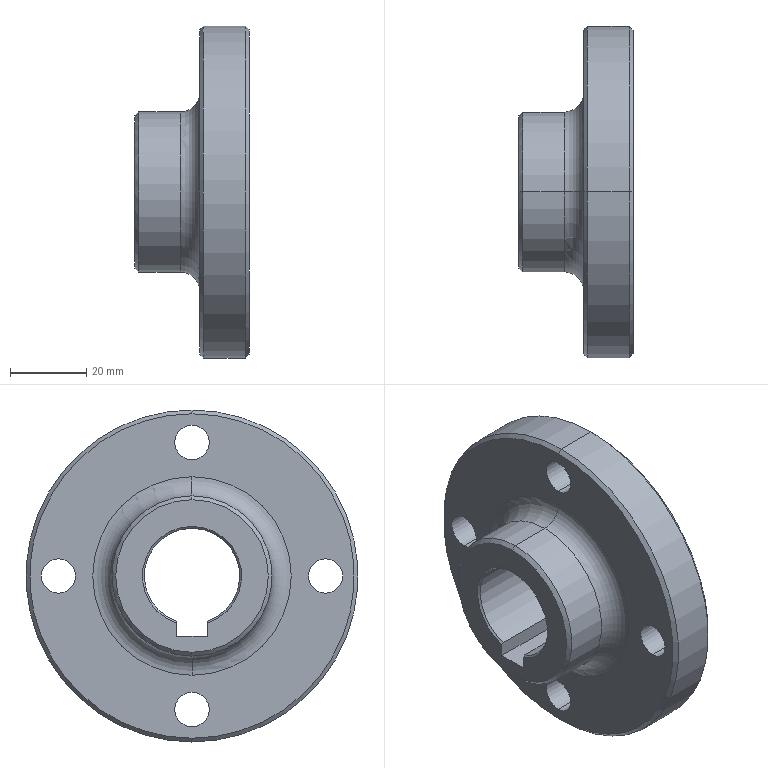Part | SolidWorks | features Chamfer 3, ICE 2, Fillet 1, Revolution 1 | 1 solid | 31 faces | box 30 x 87 x 87 mm | volume 82347 mm3 | cylinder 14 | cone 9 | plane 6 | torus 2 | commonest cylinder face diameters 9 x8 25 x2 42 x2 87 x2
STEP:
#1=CARTESIAN_POINT('',(30.,0.,-39.5));
#2=VERTEX_POINT('',#1);
#3=CARTESIAN_POINT('',(30.,0.,-30.5));
#4=VERTEX_POINT('',#3);
#5=CARTESIAN_POINT('',(30.,0.,-35.));
#6=DIRECTION('',(-1.,0.,0.));
#7=DIRECTION('',(0.,0.,1.));
#8=AXIS2_PLACEMENT_3D('',#5,#6,#7);
#9=CIRCLE('',#8,4.5);
#10=EDGE_CURVE('',#2,#4,#9,.T.);
#11=ORIENTED_EDGE('',*,*,#10,.F.);
#12=CARTESIAN_POINT('',(17.,0.,-39.5));
#13=VERTEX_POINT('',#12);
#14=CARTESIAN_POINT('',(37.,0.,-39.5));
#15=DIRECTION('',(-1.,0.,0.));
#16=VECTOR('',#15,1000.);
#17=LINE('',#14,#16);
#18=EDGE_CURVE('',#2,#13,#17,.T.);
#19=ORIENTED_EDGE('',*,*,#18,.T.);
#20=CARTESIAN_POINT('',(17.,0.,-30.5));
#21=VERTEX_POINT('',#20);
#22=CARTESIAN_POINT('',(17.,0.,-35.));
#23=DIRECTION('',(-1.,0.,0.));
#24=DIRECTION('',(0.,0.,1.));
#25=AXIS2_PLACEMENT_3D('',#22,#23,#24);
#26=CIRCLE('',#25,4.5);
#27=EDGE_CURVE('',#13,#21,#26,.T.);
#28=ORIENTED_EDGE('',*,*,#27,.T.);
#29=CARTESIAN_POINT('',(37.,0.,-30.5));
#30=DIRECTION('',(-1.,0.,0.));
#31=VECTOR('',#30,1000.);
#32=LINE('',#29,#31);
#33=EDGE_CURVE('',#4,#21,#32,.T.);
#34=ORIENTED_EDGE('',*,*,#33,.F.);
#35=EDGE_LOOP('',(#11,#19,#28,#34));
#36=FACE_OUTER_BOUND('',#35,.T.);
#37=CARTESIAN_POINT('',(37.,0.,-35.));
#38=DIRECTION('',(-1.,0.,0.));
#39=DIRECTION('',(0.,0.,1.));
#40=AXIS2_PLACEMENT_3D('',#37,#38,#39);
#41=CYLINDRICAL_SURFACE('',#40,4.5);
#42=ADVANCED_FACE('',(#36),#41,.F.);
#43=CARTESIAN_POINT('',(30.,35.,-4.5));
#44=VERTEX_POINT('',#43);
#45=CARTESIAN_POINT('',(30.,35.,4.5));
#46=VERTEX_POINT('',#45);
#47=CARTESIAN_POINT('',(30.,35.,0.));
#48=DIRECTION('',(-1.,0.,0.));
#49=DIRECTION('',(0.,0.,1.));
#50=AXIS2_PLACEMENT_3D('',#47,#48,#49);
#51=CIRCLE('',#50,4.5);
#52=EDGE_CURVE('',#44,#46,#51,.T.);
#53=ORIENTED_EDGE('',*,*,#52,.F.);
#54=CARTESIAN_POINT('',(17.,35.,-4.5));
#55=VERTEX_POINT('',#54);
#56=CARTESIAN_POINT('',(37.,35.,-4.5));
#57=DIRECTION('',(-1.,0.,0.));
#58=VECTOR('',#57,1000.);
#59=LINE('',#56,#58);
#60=EDGE_CURVE('',#44,#55,#59,.T.);
#61=ORIENTED_EDGE('',*,*,#60,.T.);
#62=CARTESIAN_POINT('',(17.,35.,4.5));
#63=VERTEX_POINT('',#62);
#64=CARTESIAN_POINT('',(17.,35.,0.));
#65=DIRECTION('',(-1.,0.,0.));
#66=DIRECTION('',(0.,0.,1.));
#67=AXIS2_PLACEMENT_3D('',#64,#65,#66);
#68=CIRCLE('',#67,4.5);
#69=EDGE_CURVE('',#55,#63,#68,.T.);
#70=ORIENTED_EDGE('',*,*,#69,.T.);
#71=CARTESIAN_POINT('',(37.,35.,4.5));
#72=DIRECTION('',(-1.,0.,0.));
#73=VECTOR('',#72,1000.);
#74=LINE('',#71,#73);
#75=EDGE_CURVE('',#46,#63,#74,.T.);
#76=ORIENTED_EDGE('',*,*,#75,.F.);
#77=EDGE_LOOP('',(#53,#61,#70,#76));
#78=FACE_OUTER_BOUND('',#77,.T.);
#79=CARTESIAN_POINT('',(37.,35.,0.));
#80=DIRECTION('',(-1.,0.,0.));
#81=DIRECTION('',(0.,0.,1.));
#82=AXIS2_PLACEMENT_3D('',#79,#80,#81);
#83=CYLINDRICAL_SURFACE('',#82,4.5);
#84=ADVANCED_FACE('',(#78),#83,.F.);
#85=CARTESIAN_POINT('',(30.,-35.,-4.5));
#86=VERTEX_POINT('',#85);
#87=CARTESIAN_POINT('',(30.,-35.,4.5));
#88=VERTEX_POINT('',#87);
#89=CARTESIAN_POINT('',(30.,-35.,0.));
#90=DIRECTION('',(-1.,0.,0.));
#91=DIRECTION('',(0.,0.,1.));
#92=AXIS2_PLACEMENT_3D('',#89,#90,#91);
#93=CIRCLE('',#92,4.5);
#94=EDGE_CURVE('',#86,#88,#93,.T.);
#95=ORIENTED_EDGE('',*,*,#94,.F.);
#96=CARTESIAN_POINT('',(17.,-35.,-4.5));
#97=VERTEX_POINT('',#96);
#98=CARTESIAN_POINT('',(37.,-35.,-4.5));
#99=DIRECTION('',(-1.,0.,0.));
#100=VECTOR('',#99,1000.);
#101=LINE('',#98,#100);
#102=EDGE_CURVE('',#86,#97,#101,.T.);
#103=ORIENTED_EDGE('',*,*,#102,.T.);
#104=CARTESIAN_POINT('',(17.,-35.,4.5));
#105=VERTEX_POINT('',#104);
#106=CARTESIAN_POINT('',(17.,-35.,0.));
#107=DIRECTION('',(-1.,0.,0.));
#108=DIRECTION('',(0.,0.,1.));
#109=AXIS2_PLACEMENT_3D('',#106,#107,#108);
#110=CIRCLE('',#109,4.5);
#111=EDGE_CURVE('',#97,#105,#110,.T.);
#112=ORIENTED_EDGE('',*,*,#111,.T.);
#113=CARTESIAN_POINT('',(37.,-35.,4.5));
#114=DIRECTION('',(-1.,0.,0.));
#115=VECTOR('',#114,1000.);
#116=LINE('',#113,#115);
#117=EDGE_CURVE('',#88,#105,#116,.T.);
#118=ORIENTED_EDGE('',*,*,#117,.F.);
#119=EDGE_LOOP('',(#95,#103,#112,#118));
#120=FACE_OUTER_BOUND('',#119,.T.);
#121=CARTESIAN_POINT('',(37.,-35.,0.));
#122=DIRECTION('',(-1.,0.,0.));
#123=DIRECTION('',(0.,0.,1.));
#124=AXIS2_PLACEMENT_3D('',#121,#122,#123);
#125=CYLINDRICAL_SURFACE('',#124,4.5);
#126=ADVANCED_FACE('',(#120),#125,.F.);
#127=CARTESIAN_POINT('',(30.,0.,30.5));
#128=VERTEX_POINT('',#127);
#129=CARTESIAN_POINT('',(30.,0.,39.5));
#130=VERTEX_POINT('',#129);
#131=CARTESIAN_POINT('',(30.,0.,35.));
#132=DIRECTION('',(-1.,0.,0.));
#133=DIRECTION('',(0.,0.,1.));
#134=AXIS2_PLACEMENT_3D('',#131,#132,#133);
#135=CIRCLE('',#134,4.5);
#136=EDGE_CURVE('',#128,#130,#135,.T.);
#137=ORIENTED_EDGE('',*,*,#136,.F.);
#138=CARTESIAN_POINT('',(17.,0.,30.5));
#139=VERTEX_POINT('',#138);
#140=CARTESIAN_POINT('',(37.,0.,30.5));
#141=DIRECTION('',(-1.,0.,0.));
#142=VECTOR('',#141,1000.);
#143=LINE('',#140,#142);
#144=EDGE_CURVE('',#128,#139,#143,.T.);
#145=ORIENTED_EDGE('',*,*,#144,.T.);
#146=CARTESIAN_POINT('',(17.,0.,39.5));
#147=VERTEX_POINT('',#146);
#148=CARTESIAN_POINT('',(17.,0.,35.));
#149=DIRECTION('',(-1.,0.,0.));
#150=DIRECTION('',(0.,0.,1.));
#151=AXIS2_PLACEMENT_3D('',#148,#149,#150);
#152=CIRCLE('',#151,4.5);
#153=EDGE_CURVE('',#139,#147,#152,.T.);
#154=ORIENTED_EDGE('',*,*,#153,.T.);
#155=CARTESIAN_POINT('',(37.,0.,39.5));
#156=DIRECTION('',(-1.,0.,0.));
#157=VECTOR('',#156,1000.);
#158=LINE('',#155,#157);
#159=EDGE_CURVE('',#130,#147,#158,.T.);
#160=ORIENTED_EDGE('',*,*,#159,.F.);
#161=EDGE_LOOP('',(#137,#145,#154,#160));
#162=FACE_OUTER_BOUND('',#161,.T.);
#163=CARTESIAN_POINT('',(37.,0.,35.));
#164=DIRECTION('',(-1.,0.,0.));
#165=DIRECTION('',(0.,0.,1.));
#166=AXIS2_PLACEMENT_3D('',#163,#164,#165);
#167=CYLINDRICAL_SURFACE('',#166,4.5);
#168=ADVANCED_FACE('',(#162),#167,.F.);
#169=CARTESIAN_POINT('',(17.,0.,42.5));
#170=VERTEX_POINT('',#169);
#171=CARTESIAN_POINT('',(17.,0.,-42.5));
#172=VERTEX_POINT('',#171);
#173=CARTESIAN_POINT('',(17.,0.,0.));
#174=DIRECTION('',(-1.,0.,0.));
#175=DIRECTION('',(0.,0.,-1.));
#176=AXIS2_PLACEMENT_3D('',#173,#174,#175);
#177=CIRCLE('',#176,42.5);
#178=EDGE_CURVE('',#170,#172,#177,.T.);
#179=ORIENTED_EDGE('',*,*,#178,.F.);
#180=CARTESIAN_POINT('',(18.,0.,43.5));
#181=VERTEX_POINT('',#180);
#182=CARTESIAN_POINT('',(17.,0.,42.5));
#183=DIRECTION('',(0.7071,0.,0.7071));
#184=VECTOR('',#183,1000.);
#185=LINE('',#182,#184);
#186=EDGE_CURVE('',#170,#181,#185,.T.);
#187=ORIENTED_EDGE('',*,*,#186,.T.);
#188=CARTESIAN_POINT('',(18.,0.,-43.5));
#189=VERTEX_POINT('',#188);
#190=CARTESIAN_POINT('',(18.,0.,0.));
#191=DIRECTION('',(1.,0.,0.));
#192=DIRECTION('',(0.,0.,-1.));
#193=AXIS2_PLACEMENT_3D('',#190,#191,#192);
#194=CIRCLE('',#193,43.5);
#195=EDGE_CURVE('',#189,#181,#194,.T.);
#196=ORIENTED_EDGE('',*,*,#195,.F.);
#197=CARTESIAN_POINT('',(17.,0.,-42.5));
#198=DIRECTION('',(0.7071,0.,-0.7071));
#199=VECTOR('',#198,1000.);
#200=LINE('',#197,#199);
#201=EDGE_CURVE('',#172,#189,#200,.T.);
#202=ORIENTED_EDGE('',*,*,#201,.F.);
#203=EDGE_LOOP('',(#179,#187,#196,#202));
#204=FACE_OUTER_BOUND('',#203,.T.);
#205=CARTESIAN_POINT('',(17.,0.,0.));
#206=DIRECTION('',(1.,0.,0.));
#207=DIRECTION('',(0.,0.,-1.));
#208=AXIS2_PLACEMENT_3D('',#205,#206,#207);
#209=CONICAL_SURFACE('',#208,42.5,0.7854);
#210=ADVANCED_FACE('',(#204),#209,.T.);
#211=CARTESIAN_POINT('',(30.,0.,-42.5));
#212=VERTEX_POINT('',#211);
#213=CARTESIAN_POINT('',(30.,0.,42.5));
#214=VERTEX_POINT('',#213);
#215=CARTESIAN_POINT('',(30.,0.,0.));
#216=DIRECTION('',(1.,0.,0.));
#217=DIRECTION('',(0.,0.,1.));
#218=AXIS2_PLACEMENT_3D('',#215,#216,#217);
#219=CIRCLE('',#218,42.5);
#220=EDGE_CURVE('',#212,#214,#219,.T.);
#221=ORIENTED_EDGE('',*,*,#220,.F.);
#222=CARTESIAN_POINT('',(29.,0.,-43.5));
#223=VERTEX_POINT('',#222);
#224=CARTESIAN_POINT('',(29.,0.,-43.5));
#225=DIRECTION('',(-0.7071,0.,-0.7071));
#226=VECTOR('',#225,1000.);
#227=LINE('',#224,#226);
#228=EDGE_CURVE('',#212,#223,#227,.T.);
#229=ORIENTED_EDGE('',*,*,#228,.T.);
#230=CARTESIAN_POINT('',(29.,0.,43.5));
#231=VERTEX_POINT('',#230);
#232=CARTESIAN_POINT('',(29.,0.,0.));
#233=DIRECTION('',(-1.,0.,0.));
#234=DIRECTION('',(0.,0.,1.));
#235=AXIS2_PLACEMENT_3D('',#232,#233,#234);
#236=CIRCLE('',#235,43.5);
#237=EDGE_CURVE('',#231,#223,#236,.T.);
#238=ORIENTED_EDGE('',*,*,#237,.F.);
#239=CARTESIAN_POINT('',(29.,0.,43.5));
#240=DIRECTION('',(-0.7071,0.,0.7071));
#241=VECTOR('',#240,1000.);
#242=LINE('',#239,#241);
#243=EDGE_CURVE('',#214,#231,#242,.T.);
#244=ORIENTED_EDGE('',*,*,#243,.F.);
#245=EDGE_LOOP('',(#221,#229,#238,#244));
#246=FACE_OUTER_BOUND('',#245,.T.);
#247=CARTESIAN_POINT('',(29.,0.,0.));
#248=DIRECTION('',(-1.,0.,0.));
#249=DIRECTION('',(0.,0.,1.));
#250=AXIS2_PLACEMENT_3D('',#247,#248,#249);
#251=CONICAL_SURFACE('',#250,43.5,0.7854);
#252=ADVANCED_FACE('',(#246),#251,.T.);
#253=CARTESIAN_POINT('',(17.,0.,26.));
#254=VERTEX_POINT('',#253);
#255=CARTESIAN_POINT('',(17.,0.,-26.));
#256=VERTEX_POINT('',#255);
#257=CARTESIAN_POINT('',(17.,0.,0.));
#258=DIRECTION('',(1.,0.,0.));
#259=DIRECTION('',(0.,0.,-1.));
#260=AXIS2_PLACEMENT_3D('',#257,#258,#259);
#261=CIRCLE('',#260,26.);
#262=EDGE_CURVE('',#254,#256,#261,.T.);
#263=ORIENTED_EDGE('',*,*,#262,.F.);
#264=CARTESIAN_POINT('',(12.,0.,21.));
#265=VERTEX_POINT('',#264);
#266=CARTESIAN_POINT('',(12.,0.,26.));
#267=DIRECTION('',(0.,1.,0.));
#268=DIRECTION('',(0.,0.,1.));
#269=AXIS2_PLACEMENT_3D('',#266,#267,#268);
#270=CIRCLE('',#269,5.);
#271=EDGE_CURVE('',#254,#265,#270,.T.);
#272=ORIENTED_EDGE('',*,*,#271,.T.);
#273=CARTESIAN_POINT('',(12.,0.,-21.));
#274=VERTEX_POINT('',#273);
#275=CARTESIAN_POINT('',(12.,0.,0.));
#276=DIRECTION('',(-1.,0.,0.));
#277=DIRECTION('',(0.,0.,-1.));
#278=AXIS2_PLACEMENT_3D('',#275,#276,#277);
#279=CIRCLE('',#278,21.);
#280=EDGE_CURVE('',#274,#265,#279,.T.);
#281=ORIENTED_EDGE('',*,*,#280,.F.);
#282=CARTESIAN_POINT('',(12.,0.,-26.));
#283=DIRECTION('',(0.,-1.,0.));
#284=DIRECTION('',(0.,0.,-1.));
#285=AXIS2_PLACEMENT_3D('',#282,#283,#284);
#286=CIRCLE('',#285,5.);
#287=EDGE_CURVE('',#256,#274,#286,.T.);
#288=ORIENTED_EDGE('',*,*,#287,.F.);
#289=EDGE_LOOP('',(#263,#272,#281,#288));
#290=FACE_OUTER_BOUND('',#289,.T.);
#291=CARTESIAN_POINT('',(12.,0.,0.));
#292=DIRECTION('',(1.,0.,0.));
#293=DIRECTION('',(0.,0.,-1.));
#294=AXIS2_PLACEMENT_3D('',#291,#292,#293);
#295=TOROIDAL_SURFACE('',#294,26.,5.);
#296=ADVANCED_FACE('',(#290),#295,.F.);
#297=CARTESIAN_POINT('',(0.5,0.,12.5));
#298=VERTEX_POINT('',#297);
#299=CARTESIAN_POINT('',(0.5,4.,-11.843));
#300=VERTEX_POINT('',#299);
#301=CARTESIAN_POINT('',(0.5,0.,0.));
#302=DIRECTION('',(-1.,0.,0.));
#303=DIRECTION('',(0.,0.,-1.));
#304=AXIS2_PLACEMENT_3D('',#301,#302,#303);
#305=CIRCLE('',#304,12.5);
#306=EDGE_CURVE('',#298,#300,#305,.T.);
#307=ORIENTED_EDGE('',*,*,#306,.F.);
#308=CARTESIAN_POINT('',(0.,0.,13.));
#309=VERTEX_POINT('',#308);
#310=CARTESIAN_POINT('',(0.5,0.,12.5));
#311=DIRECTION('',(-0.7071,0.,0.7071));
#312=VECTOR('',#311,1000.);
#313=LINE('',#310,#312);
#314=EDGE_CURVE('',#298,#309,#313,.T.);
#315=ORIENTED_EDGE('',*,*,#314,.T.);
#316=CARTESIAN_POINT('',(0.,4.,-12.369));
#317=VERTEX_POINT('',#316);
#318=CARTESIAN_POINT('',(0.,0.,0.));
#319=DIRECTION('',(1.,0.,0.));
#320=DIRECTION('',(0.,0.,-1.));
#321=AXIS2_PLACEMENT_3D('',#318,#319,#320);
#322=CIRCLE('',#321,13.);
#323=EDGE_CURVE('',#317,#309,#322,.T.);
#324=ORIENTED_EDGE('',*,*,#323,.F.);
#325=CARTESIAN_POINT('',(0.5,4.,-11.843));
#326=CARTESIAN_POINT('',(0.3335,4.,-12.018));
#327=CARTESIAN_POINT('',(0.1669,4.,-12.194));
#328=CARTESIAN_POINT('',(0.,4.,-12.369));
#329=B_SPLINE_CURVE_WITH_KNOTS('',3,(#325,#326,#327,#328),.UNSPECIFIED.,.F.,.F.,(4,4),(0.00787,0.008596),.UNSPECIFIED.);
#330=EDGE_CURVE('',#300,#317,#329,.T.);
#331=ORIENTED_EDGE('',*,*,#330,.F.);
#332=EDGE_LOOP('',(#307,#315,#324,#331));
#333=FACE_OUTER_BOUND('',#332,.T.);
#334=CARTESIAN_POINT('',(0.5,0.,0.));
#335=DIRECTION('',(-1.,0.,0.));
#336=DIRECTION('',(0.,0.,1.));
#337=AXIS2_PLACEMENT_3D('',#334,#335,#336);
#338=CONICAL_SURFACE('',#337,12.5,0.7854);
#339=ADVANCED_FACE('',(#333),#338,.F.);
#340=CARTESIAN_POINT('',(0.,0.,20.));
#341=VERTEX_POINT('',#340);
#342=CARTESIAN_POINT('',(0.,0.,-20.));
#343=VERTEX_POINT('',#342);
#344=CARTESIAN_POINT('',(0.,0.,0.));
#345=DIRECTION('',(-1.,0.,0.));
#346=DIRECTION('',(0.,0.,-1.));
#347=AXIS2_PLACEMENT_3D('',#344,#345,#346);
#348=CIRCLE('',#347,20.);
#349=EDGE_CURVE('',#341,#343,#348,.T.);
#350=ORIENTED_EDGE('',*,*,#349,.F.);
#351=CARTESIAN_POINT('',(1.,0.,21.));
#352=VERTEX_POINT('',#351);
#353=CARTESIAN_POINT('',(0.,0.,20.));
#354=DIRECTION('',(0.7071,0.,0.7071));
#355=VECTOR('',#354,1000.);
#356=LINE('',#353,#355);
#357=EDGE_CURVE('',#341,#352,#356,.T.);
#358=ORIENTED_EDGE('',*,*,#357,.T.);
#359=CARTESIAN_POINT('',(1.,0.,-21.));
#360=VERTEX_POINT('',#359);
#361=CARTESIAN_POINT('',(1.,0.,0.));
#362=DIRECTION('',(1.,0.,0.));
#363=DIRECTION('',(0.,0.,-1.));
#364=AXIS2_PLACEMENT_3D('',#361,#362,#363);
#365=CIRCLE('',#364,21.);
#366=EDGE_CURVE('',#360,#352,#365,.T.);
#367=ORIENTED_EDGE('',*,*,#366,.F.);
#368=CARTESIAN_POINT('',(0.,0.,-20.));
#369=DIRECTION('',(0.7071,0.,-0.7071));
#370=VECTOR('',#369,1000.);
#371=LINE('',#368,#370);
#372=EDGE_CURVE('',#343,#360,#371,.T.);
#373=ORIENTED_EDGE('',*,*,#372,.F.);
#374=EDGE_LOOP('',(#350,#358,#367,#373));
#375=FACE_OUTER_BOUND('',#374,.T.);
#376=CARTESIAN_POINT('',(0.,0.,0.));
#377=DIRECTION('',(1.,0.,0.));
#378=DIRECTION('',(0.,0.,-1.));
#379=AXIS2_PLACEMENT_3D('',#376,#377,#378);
#380=CONICAL_SURFACE('',#379,20.,0.7854);
#381=ADVANCED_FACE('',(#375),#380,.T.);
#382=ORIENTED_EDGE('',*,*,#237,.T.);
#383=CARTESIAN_POINT('',(0.,0.,-43.5));
#384=DIRECTION('',(-1.,0.,0.));
#385=VECTOR('',#384,1000.);
#386=LINE('',#383,#385);
#387=EDGE_CURVE('',#223,#189,#386,.T.);
#388=ORIENTED_EDGE('',*,*,#387,.T.);
#389=ORIENTED_EDGE('',*,*,#195,.T.);
#390=CARTESIAN_POINT('',(0.,0.,43.5));
#391=DIRECTION('',(-1.,0.,0.));
#392=VECTOR('',#391,1000.);
#393=LINE('',#390,#392);
#394=EDGE_CURVE('',#231,#181,#393,.T.);
#395=ORIENTED_EDGE('',*,*,#394,.F.);
#396=EDGE_LOOP('',(#382,#388,#389,#395));
#397=FACE_OUTER_BOUND('',#396,.T.);
#398=CARTESIAN_POINT('',(0.,0.,0.));
#399=DIRECTION('',(-1.,0.,0.));
#400=DIRECTION('',(0.,0.,1.));
#401=AXIS2_PLACEMENT_3D('',#398,#399,#400);
#402=CYLINDRICAL_SURFACE('',#401,43.5);
#403=ADVANCED_FACE('',(#397),#402,.T.);
#404=CARTESIAN_POINT('',(29.5,4.,-11.843));
#405=VERTEX_POINT('',#404);
#406=CARTESIAN_POINT('',(29.5,0.,12.5));
#407=VERTEX_POINT('',#406);
#408=CARTESIAN_POINT('',(29.5,0.,0.));
#409=DIRECTION('',(1.,0.,0.));
#410=DIRECTION('',(0.,0.,1.));
#411=AXIS2_PLACEMENT_3D('',#408,#409,#410);
#412=CIRCLE('',#411,12.5);
#413=EDGE_CURVE('',#405,#407,#412,.T.);
#414=ORIENTED_EDGE('',*,*,#413,.T.);
#415=CARTESIAN_POINT('',(0.,0.,12.5));
#416=DIRECTION('',(-1.,0.,0.));
#417=VECTOR('',#416,1000.);
#418=LINE('',#415,#417);
#419=EDGE_CURVE('',#407,#298,#418,.T.);
#420=ORIENTED_EDGE('',*,*,#419,.T.);
#421=ORIENTED_EDGE('',*,*,#306,.T.);
#422=CARTESIAN_POINT('',(0.,4.,-11.843));
#423=DIRECTION('',(1.,0.,0.));
#424=VECTOR('',#423,1000.);
#425=LINE('',#422,#424);
#426=EDGE_CURVE('',#300,#405,#425,.T.);
#427=ORIENTED_EDGE('',*,*,#426,.T.);
#428=EDGE_LOOP('',(#414,#420,#421,#427));
#429=FACE_OUTER_BOUND('',#428,.T.);
#430=CARTESIAN_POINT('',(0.,0.,0.));
#431=DIRECTION('',(-1.,0.,0.));
#432=DIRECTION('',(0.,0.,1.));
#433=AXIS2_PLACEMENT_3D('',#430,#431,#432);
#434=CYLINDRICAL_SURFACE('',#433,12.5);
#435=ADVANCED_FACE('',(#429),#434,.F.);
#436=CARTESIAN_POINT('',(12.,0.,0.));
#437=DIRECTION('',(-1.,0.,0.));
#438=DIRECTION('',(0.,0.,-1.));
#439=AXIS2_PLACEMENT_3D('',#436,#437,#438);
#440=CIRCLE('',#439,21.);
#441=EDGE_CURVE('',#265,#274,#440,.T.);
#442=ORIENTED_EDGE('',*,*,#441,.T.);
#443=CARTESIAN_POINT('',(0.,0.,-21.));
#444=DIRECTION('',(-1.,0.,0.));
#445=VECTOR('',#444,1000.);
#446=LINE('',#443,#445);
#447=EDGE_CURVE('',#274,#360,#446,.T.);
#448=ORIENTED_EDGE('',*,*,#447,.T.);
#449=ORIENTED_EDGE('',*,*,#366,.T.);
#450=CARTESIAN_POINT('',(0.,0.,21.));
#451=DIRECTION('',(-1.,0.,0.));
#452=VECTOR('',#451,1000.);
#453=LINE('',#450,#452);
#454=EDGE_CURVE('',#265,#352,#453,.T.);
#455=ORIENTED_EDGE('',*,*,#454,.F.);
#456=EDGE_LOOP('',(#442,#448,#449,#455));
#457=FACE_OUTER_BOUND('',#456,.T.);
#458=CARTESIAN_POINT('',(0.,0.,0.));
#459=DIRECTION('',(-1.,0.,0.));
#460=DIRECTION('',(0.,0.,1.));
#461=AXIS2_PLACEMENT_3D('',#458,#459,#460);
#462=CYLINDRICAL_SURFACE('',#461,21.);
#463=ADVANCED_FACE('',(#457),#462,.T.);
#464=ORIENTED_EDGE('',*,*,#447,.F.);
#465=ORIENTED_EDGE('',*,*,#280,.T.);
#466=ORIENTED_EDGE('',*,*,#454,.T.);
#467=CARTESIAN_POINT('',(1.,0.,0.));
#468=DIRECTION('',(1.,0.,0.));
#469=DIRECTION('',(0.,0.,-1.));
#470=AXIS2_PLACEMENT_3D('',#467,#468,#469);
#471=CIRCLE('',#470,21.);
#472=EDGE_CURVE('',#352,#360,#471,.T.);
#473=ORIENTED_EDGE('',*,*,#472,.T.);
#474=EDGE_LOOP('',(#464,#465,#466,#473));
#475=FACE_OUTER_BOUND('',#474,.T.);
#476=CARTESIAN_POINT('',(0.,0.,0.));
#477=DIRECTION('',(-1.,0.,0.));
#478=DIRECTION('',(0.,0.,1.));
#479=AXIS2_PLACEMENT_3D('',#476,#477,#478);
#480=CYLINDRICAL_SURFACE('',#479,21.);
#481=ADVANCED_FACE('',(#475),#480,.T.);
#482=ORIENTED_EDGE('',*,*,#323,.T.);
#483=CARTESIAN_POINT('',(0.,-4.,-12.369));
#484=VERTEX_POINT('',#483);
#485=CARTESIAN_POINT('',(0.,0.,0.));
#486=DIRECTION('',(1.,0.,0.));
#487=DIRECTION('',(0.,0.,-1.));
#488=AXIS2_PLACEMENT_3D('',#485,#486,#487);
#489=CIRCLE('',#488,13.);
#490=EDGE_CURVE('',#309,#484,#489,.T.);
#491=ORIENTED_EDGE('',*,*,#490,.T.);
#492=CARTESIAN_POINT('',(0.,-4.,-15.8));
#493=VERTEX_POINT('',#492);
#494=CARTESIAN_POINT('',(0.,-4.,-15.8));
#495=DIRECTION('',(0.,0.,-1.));
#496=VECTOR('',#495,1000.);
#497=LINE('',#494,#496);
#498=EDGE_CURVE('',#484,#493,#497,.T.);
#499=ORIENTED_EDGE('',*,*,#498,.T.);
#500=CARTESIAN_POINT('',(0.,4.,-15.8));
#501=VERTEX_POINT('',#500);
#502=CARTESIAN_POINT('',(0.,4.,-15.8));
#503=DIRECTION('',(0.,1.,0.));
#504=VECTOR('',#503,1000.);
#505=LINE('',#502,#504);
#506=EDGE_CURVE('',#493,#501,#505,.T.);
#507=ORIENTED_EDGE('',*,*,#506,.T.);
#508=CARTESIAN_POINT('',(0.,4.,-15.8));
#509=DIRECTION('',(0.,0.,1.));
#510=VECTOR('',#509,1000.);
#511=LINE('',#508,#510);
#512=EDGE_CURVE('',#501,#317,#511,.T.);
#513=ORIENTED_EDGE('',*,*,#512,.T.);
#514=EDGE_LOOP('',(#482,#491,#499,#507,#513));
#515=FACE_BOUND('',#514,.T.);
#516=CARTESIAN_POINT('',(0.,0.,0.));
#517=DIRECTION('',(-1.,0.,0.));
#518=DIRECTION('',(0.,0.,-1.));
#519=AXIS2_PLACEMENT_3D('',#516,#517,#518);
#520=CIRCLE('',#519,20.);
#521=EDGE_CURVE('',#343,#341,#520,.T.);
#522=ORIENTED_EDGE('',*,*,#521,.T.);
#523=ORIENTED_EDGE('',*,*,#349,.T.);
#524=EDGE_LOOP('',(#522,#523));
#525=FACE_OUTER_BOUND('',#524,.T.);
#526=CARTESIAN_POINT('',(0.,12.5,0.));
#527=DIRECTION('',(1.,0.,0.));
#528=DIRECTION('',(0.,0.,-1.));
#529=AXIS2_PLACEMENT_3D('',#526,#527,#528);
#530=PLANE('',#529);
#531=ADVANCED_FACE('',(#515,#525),#530,.F.);
#532=ORIENTED_EDGE('',*,*,#419,.F.);
#533=CARTESIAN_POINT('',(29.5,-4.,-11.843));
#534=VERTEX_POINT('',#533);
#535=CARTESIAN_POINT('',(29.5,0.,0.));
#536=DIRECTION('',(1.,0.,0.));
#537=DIRECTION('',(0.,0.,1.));
#538=AXIS2_PLACEMENT_3D('',#535,#536,#537);
#539=CIRCLE('',#538,12.5);
#540=EDGE_CURVE('',#407,#534,#539,.T.);
#541=ORIENTED_EDGE('',*,*,#540,.T.);
#542=CARTESIAN_POINT('',(0.5,-4.,-11.843));
#543=VERTEX_POINT('',#542);
#544=CARTESIAN_POINT('',(0.,-4.,-11.843));
#545=DIRECTION('',(-1.,0.,0.));
#546=VECTOR('',#545,1000.);
#547=LINE('',#544,#546);
#548=EDGE_CURVE('',#534,#543,#547,.T.);
#549=ORIENTED_EDGE('',*,*,#548,.T.);
#550=CARTESIAN_POINT('',(0.5,0.,0.));
#551=DIRECTION('',(-1.,0.,0.));
#552=DIRECTION('',(0.,0.,-1.));
#553=AXIS2_PLACEMENT_3D('',#550,#551,#552);
#554=CIRCLE('',#553,12.5);
#555=EDGE_CURVE('',#543,#298,#554,.T.);
#556=ORIENTED_EDGE('',*,*,#555,.T.);
#557=EDGE_LOOP('',(#532,#541,#549,#556));
#558=FACE_OUTER_BOUND('',#557,.T.);
#559=CARTESIAN_POINT('',(0.,0.,0.));
#560=DIRECTION('',(-1.,0.,0.));
#561=DIRECTION('',(0.,0.,1.));
#562=AXIS2_PLACEMENT_3D('',#559,#560,#561);
#563=CYLINDRICAL_SURFACE('',#562,12.5);
#564=ADVANCED_FACE('',(#558),#563,.F.);
#565=CARTESIAN_POINT('',(30.,0.,-35.));
#566=DIRECTION('',(-1.,0.,0.));
#567=DIRECTION('',(0.,0.,1.));
#568=AXIS2_PLACEMENT_3D('',#565,#566,#567);
#569=CIRCLE('',#568,4.5);
#570=EDGE_CURVE('',#4,#2,#569,.T.);
#571=ORIENTED_EDGE('',*,*,#570,.T.);
#572=ORIENTED_EDGE('',*,*,#10,.T.);
#573=EDGE_LOOP('',(#571,#572));
#574=FACE_BOUND('',#573,.T.);
#575=CARTESIAN_POINT('',(30.,35.,0.));
#576=DIRECTION('',(-1.,0.,0.));
#577=DIRECTION('',(0.,0.,1.));
#578=AXIS2_PLACEMENT_3D('',#575,#576,#577);
#579=CIRCLE('',#578,4.5);
#580=EDGE_CURVE('',#46,#44,#579,.T.);
#581=ORIENTED_EDGE('',*,*,#580,.T.);
#582=ORIENTED_EDGE('',*,*,#52,.T.);
#583=EDGE_LOOP('',(#581,#582));
#584=FACE_BOUND('',#583,.T.);
#585=CARTESIAN_POINT('',(30.,-35.,0.));
#586=DIRECTION('',(-1.,0.,0.));
#587=DIRECTION('',(0.,0.,1.));
#588=AXIS2_PLACEMENT_3D('',#585,#586,#587);
#589=CIRCLE('',#588,4.5);
#590=EDGE_CURVE('',#88,#86,#589,.T.);
#591=ORIENTED_EDGE('',*,*,#590,.T.);
#592=ORIENTED_EDGE('',*,*,#94,.T.);
#593=EDGE_LOOP('',(#591,#592));
#594=FACE_BOUND('',#593,.T.);
#595=CARTESIAN_POINT('',(30.,0.,35.));
#596=DIRECTION('',(-1.,0.,0.));
#597=DIRECTION('',(0.,0.,1.));
#598=AXIS2_PLACEMENT_3D('',#595,#596,#597);
#599=CIRCLE('',#598,4.5);
#600=EDGE_CURVE('',#130,#128,#599,.T.);
#601=ORIENTED_EDGE('',*,*,#600,.T.);
#602=ORIENTED_EDGE('',*,*,#136,.T.);
#603=EDGE_LOOP('',(#601,#602));
#604=FACE_BOUND('',#603,.T.);
#605=CARTESIAN_POINT('',(30.,0.,0.));
#606=DIRECTION('',(1.,0.,0.));
#607=DIRECTION('',(0.,0.,1.));
#608=AXIS2_PLACEMENT_3D('',#605,#606,#607);
#609=CIRCLE('',#608,42.5);
#610=EDGE_CURVE('',#214,#212,#609,.T.);
#611=ORIENTED_EDGE('',*,*,#610,.T.);
#612=ORIENTED_EDGE('',*,*,#220,.T.);
#613=EDGE_LOOP('',(#611,#612));
#614=FACE_OUTER_BOUND('',#613,.T.);
#615=CARTESIAN_POINT('',(30.,-4.,-15.8));
#616=VERTEX_POINT('',#615);
#617=CARTESIAN_POINT('',(30.,4.,-15.8));
#618=VERTEX_POINT('',#617);
#619=CARTESIAN_POINT('',(30.,4.,-15.8));
#620=DIRECTION('',(0.,1.,0.));
#621=VECTOR('',#620,1000.);
#622=LINE('',#619,#621);
#623=EDGE_CURVE('',#616,#618,#622,.T.);
#624=ORIENTED_EDGE('',*,*,#623,.F.);
#625=CARTESIAN_POINT('',(30.,-4.,-12.369));
#626=VERTEX_POINT('',#625);
#627=CARTESIAN_POINT('',(30.,-4.,-15.8));
#628=DIRECTION('',(0.,0.,-1.));
#629=VECTOR('',#628,1000.);
#630=LINE('',#627,#629);
#631=EDGE_CURVE('',#626,#616,#630,.T.);
#632=ORIENTED_EDGE('',*,*,#631,.F.);
#633=CARTESIAN_POINT('',(30.,4.,-12.369));
#634=VERTEX_POINT('',#633);
#635=CARTESIAN_POINT('',(30.,0.,0.));
#636=DIRECTION('',(-1.,0.,0.));
#637=DIRECTION('',(0.,0.,1.));
#638=AXIS2_PLACEMENT_3D('',#635,#636,#637);
#639=CIRCLE('',#638,13.);
#640=EDGE_CURVE('',#626,#634,#639,.T.);
#641=ORIENTED_EDGE('',*,*,#640,.T.);
#642=CARTESIAN_POINT('',(30.,4.,-15.8));
#643=DIRECTION('',(0.,0.,1.));
#644=VECTOR('',#643,1000.);
#645=LINE('',#642,#644);
#646=EDGE_CURVE('',#618,#634,#645,.T.);
#647=ORIENTED_EDGE('',*,*,#646,.F.);
#648=EDGE_LOOP('',(#624,#632,#641,#647));
#649=FACE_BOUND('',#648,.T.);
#650=CARTESIAN_POINT('',(30.,43.5,0.));
#651=DIRECTION('',(-1.,0.,0.));
#652=DIRECTION('',(0.,0.,1.));
#653=AXIS2_PLACEMENT_3D('',#650,#651,#652);
#654=PLANE('',#653);
#655=ADVANCED_FACE('',(#574,#584,#594,#604,#614,#649),#654,.F.);
#656=ORIENTED_EDGE('',*,*,#387,.F.);
#657=CARTESIAN_POINT('',(29.,0.,0.));
#658=DIRECTION('',(-1.,0.,0.));
#659=DIRECTION('',(0.,0.,1.));
#660=AXIS2_PLACEMENT_3D('',#657,#658,#659);
#661=CIRCLE('',#660,43.5);
#662=EDGE_CURVE('',#223,#231,#661,.T.);
#663=ORIENTED_EDGE('',*,*,#662,.T.);
#664=ORIENTED_EDGE('',*,*,#394,.T.);
#665=CARTESIAN_POINT('',(18.,0.,0.));
#666=DIRECTION('',(1.,0.,0.));
#667=DIRECTION('',(0.,0.,-1.));
#668=AXIS2_PLACEMENT_3D('',#665,#666,#667);
#669=CIRCLE('',#668,43.5);
#670=EDGE_CURVE('',#181,#189,#669,.T.);
#671=ORIENTED_EDGE('',*,*,#670,.T.);
#672=EDGE_LOOP('',(#656,#663,#664,#671));
#673=FACE_OUTER_BOUND('',#672,.T.);
#674=CARTESIAN_POINT('',(0.,0.,0.));
#675=DIRECTION('',(-1.,0.,0.));
#676=DIRECTION('',(0.,0.,1.));
#677=AXIS2_PLACEMENT_3D('',#674,#675,#676);
#678=CYLINDRICAL_SURFACE('',#677,43.5);
#679=ADVANCED_FACE('',(#673),#678,.T.);
#680=CARTESIAN_POINT('',(17.,0.,-35.));
#681=DIRECTION('',(-1.,0.,0.));
#682=DIRECTION('',(0.,0.,1.));
#683=AXIS2_PLACEMENT_3D('',#680,#681,#682);
#684=CIRCLE('',#683,4.5);
#685=EDGE_CURVE('',#21,#13,#684,.T.);
#686=ORIENTED_EDGE('',*,*,#685,.F.);
#687=ORIENTED_EDGE('',*,*,#27,.F.);
#688=EDGE_LOOP('',(#686,#687));
#689=FACE_BOUND('',#688,.T.);
#690=CARTESIAN_POINT('',(17.,35.,0.));
#691=DIRECTION('',(-1.,0.,0.));
#692=DIRECTION('',(0.,0.,1.));
#693=AXIS2_PLACEMENT_3D('',#690,#691,#692);
#694=CIRCLE('',#693,4.5);
#695=EDGE_CURVE('',#63,#55,#694,.T.);
#696=ORIENTED_EDGE('',*,*,#695,.F.);
#697=ORIENTED_EDGE('',*,*,#69,.F.);
#698=EDGE_LOOP('',(#696,#697));
#699=FACE_BOUND('',#698,.T.);
#700=CARTESIAN_POINT('',(17.,-35.,0.));
#701=DIRECTION('',(-1.,0.,0.));
#702=DIRECTION('',(0.,0.,1.));
#703=AXIS2_PLACEMENT_3D('',#700,#701,#702);
#704=CIRCLE('',#703,4.5);
#705=EDGE_CURVE('',#105,#97,#704,.T.);
#706=ORIENTED_EDGE('',*,*,#705,.F.);
#707=ORIENTED_EDGE('',*,*,#111,.F.);
#708=EDGE_LOOP('',(#706,#707));
#709=FACE_BOUND('',#708,.T.);
#710=CARTESIAN_POINT('',(17.,0.,35.));
#711=DIRECTION('',(-1.,0.,0.));
#712=DIRECTION('',(0.,0.,1.));
#713=AXIS2_PLACEMENT_3D('',#710,#711,#712);
#714=CIRCLE('',#713,4.5);
#715=EDGE_CURVE('',#147,#139,#714,.T.);
#716=ORIENTED_EDGE('',*,*,#715,.F.);
#717=ORIENTED_EDGE('',*,*,#153,.F.);
#718=EDGE_LOOP('',(#716,#717));
#719=FACE_BOUND('',#718,.T.);
#720=CARTESIAN_POINT('',(17.,0.,0.));
#721=DIRECTION('',(-1.,0.,0.));
#722=DIRECTION('',(0.,0.,-1.));
#723=AXIS2_PLACEMENT_3D('',#720,#721,#722);
#724=CIRCLE('',#723,42.5);
#725=EDGE_CURVE('',#172,#170,#724,.T.);
#726=ORIENTED_EDGE('',*,*,#725,.T.);
#727=ORIENTED_EDGE('',*,*,#178,.T.);
#728=EDGE_LOOP('',(#726,#727));
#729=FACE_OUTER_BOUND('',#728,.T.);
#730=CARTESIAN_POINT('',(17.,0.,0.));
#731=DIRECTION('',(1.,0.,0.));
#732=DIRECTION('',(0.,0.,-1.));
#733=AXIS2_PLACEMENT_3D('',#730,#731,#732);
#734=CIRCLE('',#733,26.);
#735=EDGE_CURVE('',#256,#254,#734,.T.);
#736=ORIENTED_EDGE('',*,*,#735,.T.);
#737=ORIENTED_EDGE('',*,*,#262,.T.);
#738=EDGE_LOOP('',(#736,#737));
#739=FACE_BOUND('',#738,.T.);
#740=CARTESIAN_POINT('',(17.,21.,0.));
#741=DIRECTION('',(1.,0.,0.));
#742=DIRECTION('',(0.,0.,-1.));
#743=AXIS2_PLACEMENT_3D('',#740,#741,#742);
#744=PLANE('',#743);
#745=ADVANCED_FACE('',(#689,#699,#709,#719,#729,#739),#744,.F.);
#746=ORIENTED_EDGE('',*,*,#357,.F.);
#747=ORIENTED_EDGE('',*,*,#521,.F.);
#748=ORIENTED_EDGE('',*,*,#372,.T.);
#749=ORIENTED_EDGE('',*,*,#472,.F.);
#750=EDGE_LOOP('',(#746,#747,#748,#749));
#751=FACE_OUTER_BOUND('',#750,.T.);
#752=CARTESIAN_POINT('',(0.,0.,0.));
#753=DIRECTION('',(1.,0.,0.));
#754=DIRECTION('',(0.,0.,-1.));
#755=AXIS2_PLACEMENT_3D('',#752,#753,#754);
#756=CONICAL_SURFACE('',#755,20.,0.7854);
#757=ADVANCED_FACE('',(#751),#756,.T.);
#758=CARTESIAN_POINT('',(29.5,-4.,-11.843));
#759=CARTESIAN_POINT('',(29.666,-4.,-12.018));
#760=CARTESIAN_POINT('',(29.833,-4.,-12.194));
#761=CARTESIAN_POINT('',(30.,-4.,-12.369));
#762=B_SPLINE_CURVE_WITH_KNOTS('',3,(#758,#759,#760,#761),.UNSPECIFIED.,.F.,.F.,(4,4),(0.00787,0.008596),.UNSPECIFIED.);
#763=EDGE_CURVE('',#534,#626,#762,.T.);
#764=ORIENTED_EDGE('',*,*,#763,.F.);
#765=ORIENTED_EDGE('',*,*,#540,.F.);
#766=ORIENTED_EDGE('',*,*,#413,.F.);
#767=CARTESIAN_POINT('',(30.,4.,-12.369));
#768=CARTESIAN_POINT('',(29.833,4.,-12.194));
#769=CARTESIAN_POINT('',(29.666,4.,-12.018));
#770=CARTESIAN_POINT('',(29.5,4.,-11.843));
#771=B_SPLINE_CURVE_WITH_KNOTS('',3,(#767,#768,#769,#770),.UNSPECIFIED.,.F.,.F.,(4,4),(0.007603,0.008329),.UNSPECIFIED.);
#772=EDGE_CURVE('',#634,#405,#771,.T.);
#773=ORIENTED_EDGE('',*,*,#772,.F.);
#774=ORIENTED_EDGE('',*,*,#640,.F.);
#775=EDGE_LOOP('',(#764,#765,#766,#773,#774));
#776=FACE_OUTER_BOUND('',#775,.T.);
#777=CARTESIAN_POINT('',(30.,0.,0.));
#778=DIRECTION('',(1.,0.,0.));
#779=DIRECTION('',(0.,0.,-1.));
#780=AXIS2_PLACEMENT_3D('',#777,#778,#779);
#781=CONICAL_SURFACE('',#780,13.,0.7854);
#782=ADVANCED_FACE('',(#776),#781,.F.);
#783=ORIENTED_EDGE('',*,*,#314,.F.);
#784=ORIENTED_EDGE('',*,*,#555,.F.);
#785=CARTESIAN_POINT('',(0.,-4.,-12.369));
#786=CARTESIAN_POINT('',(0.1669,-4.,-12.194));
#787=CARTESIAN_POINT('',(0.3335,-4.,-12.018));
#788=CARTESIAN_POINT('',(0.5,-4.,-11.843));
#789=B_SPLINE_CURVE_WITH_KNOTS('',3,(#785,#786,#787,#788),.UNSPECIFIED.,.F.,.F.,(4,4),(0.007603,0.008329),.UNSPECIFIED.);
#790=EDGE_CURVE('',#484,#543,#789,.T.);
#791=ORIENTED_EDGE('',*,*,#790,.F.);
#792=ORIENTED_EDGE('',*,*,#490,.F.);
#793=EDGE_LOOP('',(#783,#784,#791,#792));
#794=FACE_OUTER_BOUND('',#793,.T.);
#795=CARTESIAN_POINT('',(0.5,0.,0.));
#796=DIRECTION('',(-1.,0.,0.));
#797=DIRECTION('',(0.,0.,1.));
#798=AXIS2_PLACEMENT_3D('',#795,#796,#797);
#799=CONICAL_SURFACE('',#798,12.5,0.7854);
#800=ADVANCED_FACE('',(#794),#799,.F.);
#801=ORIENTED_EDGE('',*,*,#271,.F.);
#802=ORIENTED_EDGE('',*,*,#735,.F.);
#803=ORIENTED_EDGE('',*,*,#287,.T.);
#804=ORIENTED_EDGE('',*,*,#441,.F.);
#805=EDGE_LOOP('',(#801,#802,#803,#804));
#806=FACE_OUTER_BOUND('',#805,.T.);
#807=CARTESIAN_POINT('',(12.,0.,0.));
#808=DIRECTION('',(1.,0.,0.));
#809=DIRECTION('',(0.,0.,-1.));
#810=AXIS2_PLACEMENT_3D('',#807,#808,#809);
#811=TOROIDAL_SURFACE('',#810,26.,5.);
#812=ADVANCED_FACE('',(#806),#811,.F.);
#813=ORIENTED_EDGE('',*,*,#228,.F.);
#814=ORIENTED_EDGE('',*,*,#610,.F.);
#815=ORIENTED_EDGE('',*,*,#243,.T.);
#816=ORIENTED_EDGE('',*,*,#662,.F.);
#817=EDGE_LOOP('',(#813,#814,#815,#816));
#818=FACE_OUTER_BOUND('',#817,.T.);
#819=CARTESIAN_POINT('',(29.,0.,0.));
#820=DIRECTION('',(-1.,0.,0.));
#821=DIRECTION('',(0.,0.,1.));
#822=AXIS2_PLACEMENT_3D('',#819,#820,#821);
#823=CONICAL_SURFACE('',#822,43.5,0.7854);
#824=ADVANCED_FACE('',(#818),#823,.T.);
#825=ORIENTED_EDGE('',*,*,#186,.F.);
#826=ORIENTED_EDGE('',*,*,#725,.F.);
#827=ORIENTED_EDGE('',*,*,#201,.T.);
#828=ORIENTED_EDGE('',*,*,#670,.F.);
#829=EDGE_LOOP('',(#825,#826,#827,#828));
#830=FACE_OUTER_BOUND('',#829,.T.);
#831=CARTESIAN_POINT('',(17.,0.,0.));
#832=DIRECTION('',(1.,0.,0.));
#833=DIRECTION('',(0.,0.,-1.));
#834=AXIS2_PLACEMENT_3D('',#831,#832,#833);
#835=CONICAL_SURFACE('',#834,42.5,0.7854);
#836=ADVANCED_FACE('',(#830),#835,.T.);
#837=ORIENTED_EDGE('',*,*,#144,.F.);
#838=ORIENTED_EDGE('',*,*,#600,.F.);
#839=ORIENTED_EDGE('',*,*,#159,.T.);
#840=ORIENTED_EDGE('',*,*,#715,.T.);
#841=EDGE_LOOP('',(#837,#838,#839,#840));
#842=FACE_OUTER_BOUND('',#841,.T.);
#843=CARTESIAN_POINT('',(37.,0.,35.));
#844=DIRECTION('',(-1.,0.,0.));
#845=DIRECTION('',(0.,0.,1.));
#846=AXIS2_PLACEMENT_3D('',#843,#844,#845);
#847=CYLINDRICAL_SURFACE('',#846,4.5);
#848=ADVANCED_FACE('',(#842),#847,.F.);
#849=ORIENTED_EDGE('',*,*,#102,.F.);
#850=ORIENTED_EDGE('',*,*,#590,.F.);
#851=ORIENTED_EDGE('',*,*,#117,.T.);
#852=ORIENTED_EDGE('',*,*,#705,.T.);
#853=EDGE_LOOP('',(#849,#850,#851,#852));
#854=FACE_OUTER_BOUND('',#853,.T.);
#855=CARTESIAN_POINT('',(37.,-35.,0.));
#856=DIRECTION('',(-1.,0.,0.));
#857=DIRECTION('',(0.,0.,1.));
#858=AXIS2_PLACEMENT_3D('',#855,#856,#857);
#859=CYLINDRICAL_SURFACE('',#858,4.5);
#860=ADVANCED_FACE('',(#854),#859,.F.);
#861=ORIENTED_EDGE('',*,*,#60,.F.);
#862=ORIENTED_EDGE('',*,*,#580,.F.);
#863=ORIENTED_EDGE('',*,*,#75,.T.);
#864=ORIENTED_EDGE('',*,*,#695,.T.);
#865=EDGE_LOOP('',(#861,#862,#863,#864));
#866=FACE_OUTER_BOUND('',#865,.T.);
#867=CARTESIAN_POINT('',(37.,35.,0.));
#868=DIRECTION('',(-1.,0.,0.));
#869=DIRECTION('',(0.,0.,1.));
#870=AXIS2_PLACEMENT_3D('',#867,#868,#869);
#871=CYLINDRICAL_SURFACE('',#870,4.5);
#872=ADVANCED_FACE('',(#866),#871,.F.);
#873=ORIENTED_EDGE('',*,*,#18,.F.);
#874=ORIENTED_EDGE('',*,*,#570,.F.);
#875=ORIENTED_EDGE('',*,*,#33,.T.);
#876=ORIENTED_EDGE('',*,*,#685,.T.);
#877=EDGE_LOOP('',(#873,#874,#875,#876));
#878=FACE_OUTER_BOUND('',#877,.T.);
#879=CARTESIAN_POINT('',(37.,0.,-35.));
#880=DIRECTION('',(-1.,0.,0.));
#881=DIRECTION('',(0.,0.,1.));
#882=AXIS2_PLACEMENT_3D('',#879,#880,#881);
#883=CYLINDRICAL_SURFACE('',#882,4.5);
#884=ADVANCED_FACE('',(#878),#883,.F.);
#885=ORIENTED_EDGE('',*,*,#623,.T.);
#886=CARTESIAN_POINT('',(0.,4.,-15.8));
#887=DIRECTION('',(1.,0.,0.));
#888=VECTOR('',#887,1000.);
#889=LINE('',#886,#888);
#890=EDGE_CURVE('',#501,#618,#889,.T.);
#891=ORIENTED_EDGE('',*,*,#890,.F.);
#892=ORIENTED_EDGE('',*,*,#506,.F.);
#893=CARTESIAN_POINT('',(0.,-4.,-15.8));
#894=DIRECTION('',(1.,0.,0.));
#895=VECTOR('',#894,1000.);
#896=LINE('',#893,#895);
#897=EDGE_CURVE('',#493,#616,#896,.T.);
#898=ORIENTED_EDGE('',*,*,#897,.T.);
#899=EDGE_LOOP('',(#885,#891,#892,#898));
#900=FACE_OUTER_BOUND('',#899,.T.);
#901=CARTESIAN_POINT('',(0.,4.,-15.8));
#902=DIRECTION('',(0.,0.,-1.));
#903=DIRECTION('',(-1.,0.,0.));
#904=AXIS2_PLACEMENT_3D('',#901,#902,#903);
#905=PLANE('',#904);
#906=ADVANCED_FACE('',(#900),#905,.F.);
#907=ORIENTED_EDGE('',*,*,#763,.T.);
#908=ORIENTED_EDGE('',*,*,#631,.T.);
#909=ORIENTED_EDGE('',*,*,#897,.F.);
#910=ORIENTED_EDGE('',*,*,#498,.F.);
#911=ORIENTED_EDGE('',*,*,#790,.T.);
#912=ORIENTED_EDGE('',*,*,#548,.F.);
#913=EDGE_LOOP('',(#907,#908,#909,#910,#911,#912));
#914=FACE_OUTER_BOUND('',#913,.T.);
#915=CARTESIAN_POINT('',(0.,-4.,-15.8));
#916=DIRECTION('',(0.,-1.,0.));
#917=DIRECTION('',(0.,0.,-1.));
#918=AXIS2_PLACEMENT_3D('',#915,#916,#917);
#919=PLANE('',#918);
#920=ADVANCED_FACE('',(#914),#919,.F.);
#921=ORIENTED_EDGE('',*,*,#772,.T.);
#922=ORIENTED_EDGE('',*,*,#426,.F.);
#923=ORIENTED_EDGE('',*,*,#330,.T.);
#924=ORIENTED_EDGE('',*,*,#512,.F.);
#925=ORIENTED_EDGE('',*,*,#890,.T.);
#926=ORIENTED_EDGE('',*,*,#646,.T.);
#927=EDGE_LOOP('',(#921,#922,#923,#924,#925,#926));
#928=FACE_OUTER_BOUND('',#927,.T.);
#929=CARTESIAN_POINT('',(0.,4.,-15.8));
#930=DIRECTION('',(0.,1.,0.));
#931=DIRECTION('',(0.,0.,1.));
#932=AXIS2_PLACEMENT_3D('',#929,#930,#931);
#933=PLANE('',#932);
#934=ADVANCED_FACE('',(#928),#933,.F.);
#935=CLOSED_SHELL('',(#42,#84,#126,#168,#210,#252,#296,#339,#381,#403,#435,#463,#481,#531,#564,#655,#679,#745,#757,#782,#800,#812,#824,#836,#848,#860,#872,#884,#906,#920,#934));
#936=MANIFOLD_SOLID_BREP('',#935);
#937=CARTESIAN_POINT('',(0.,0.,0.));
#938=DIRECTION('',(0.,0.,1.));
#939=DIRECTION('',(1.,0.,0.));
#940=AXIS2_PLACEMENT_3D('',#937,#938,#939);
#941=(LENGTH_UNIT()NAMED_UNIT(*)SI_UNIT(.MILLI.,.METRE.));
#942=UNCERTAINTY_MEASURE_WITH_UNIT(LENGTH_MEASURE(0.00001),#941,'','');
#943=(NAMED_UNIT(*)PLANE_ANGLE_UNIT()SI_UNIT($,.RADIAN.));
#944=(NAMED_UNIT(*)SI_UNIT($,.STERADIAN.)SOLID_ANGLE_UNIT());
#945=(GEOMETRIC_REPRESENTATION_CONTEXT(3)GLOBAL_UNCERTAINTY_ASSIGNED_CONTEXT((#942))GLOBAL_UNIT_ASSIGNED_CONTEXT((#941,#943,#944))REPRESENTATION_CONTEXT('',''));
#946=ADVANCED_BREP_SHAPE_REPRESENTATION('',(#936,#940),#945);